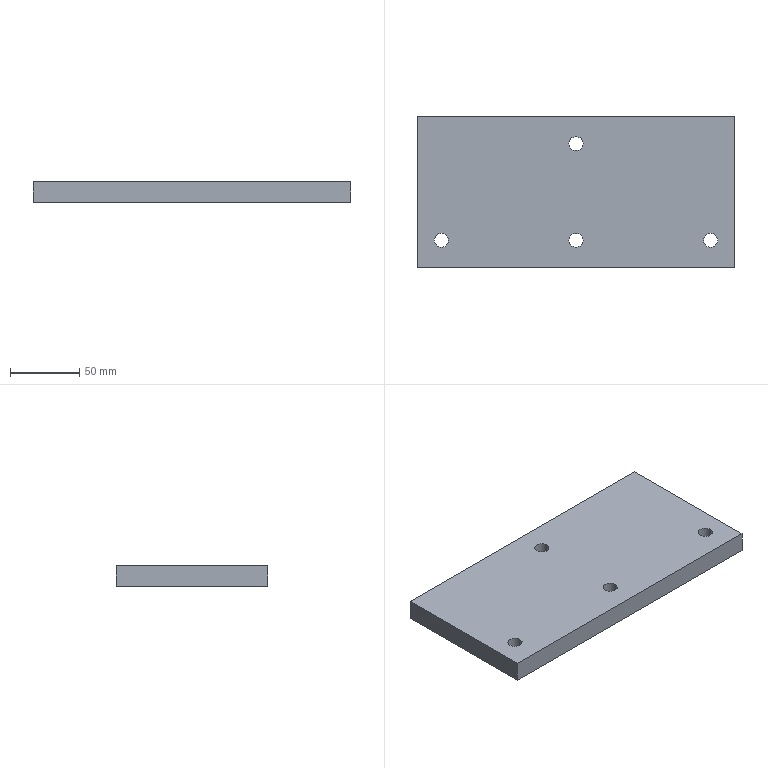Part | SolidWorks | features Extrusion 1, HoleWzd 1 | 1 solid | 14 faces | box 230 x 110 x 15 mm | volume 374597 mm3 | cylinder 8 | plane 6 | commonest cylinder face diameters 10.2 x8
STEP:
#1=CARTESIAN_POINT('',(-102.6,-35.,0.));
#2=VERTEX_POINT('',#1);
#3=CARTESIAN_POINT('',(-92.4,-35.,0.));
#4=VERTEX_POINT('',#3);
#5=CARTESIAN_POINT('',(-97.5,-35.,0.));
#6=DIRECTION('',(0.,0.,1.));
#7=DIRECTION('',(1.,0.,0.));
#8=AXIS2_PLACEMENT_3D('',#5,#6,#7);
#9=CIRCLE('',#8,5.1);
#10=EDGE_CURVE('',#2,#4,#9,.T.);
#11=ORIENTED_EDGE('',*,*,#10,.F.);
#12=CARTESIAN_POINT('',(-102.6,-35.,15.));
#13=VERTEX_POINT('',#12);
#14=CARTESIAN_POINT('',(-102.6,-35.,15.));
#15=DIRECTION('',(0.,0.,1.));
#16=VECTOR('',#15,1000.);
#17=LINE('',#14,#16);
#18=EDGE_CURVE('',#2,#13,#17,.T.);
#19=ORIENTED_EDGE('',*,*,#18,.T.);
#20=CARTESIAN_POINT('',(-92.4,-35.,15.));
#21=VERTEX_POINT('',#20);
#22=CARTESIAN_POINT('',(-97.5,-35.,15.));
#23=DIRECTION('',(0.,0.,1.));
#24=DIRECTION('',(1.,0.,0.));
#25=AXIS2_PLACEMENT_3D('',#22,#23,#24);
#26=CIRCLE('',#25,5.1);
#27=EDGE_CURVE('',#13,#21,#26,.T.);
#28=ORIENTED_EDGE('',*,*,#27,.T.);
#29=CARTESIAN_POINT('',(-92.4,-35.,15.));
#30=DIRECTION('',(0.,0.,1.));
#31=VECTOR('',#30,1000.);
#32=LINE('',#29,#31);
#33=EDGE_CURVE('',#4,#21,#32,.T.);
#34=ORIENTED_EDGE('',*,*,#33,.F.);
#35=EDGE_LOOP('',(#11,#19,#28,#34));
#36=FACE_OUTER_BOUND('',#35,.T.);
#37=CARTESIAN_POINT('',(-97.5,-35.,15.));
#38=DIRECTION('',(0.,0.,1.));
#39=DIRECTION('',(1.,0.,0.));
#40=AXIS2_PLACEMENT_3D('',#37,#38,#39);
#41=CYLINDRICAL_SURFACE('',#40,5.1);
#42=ADVANCED_FACE('',(#36),#41,.F.);
#43=CARTESIAN_POINT('',(92.4,-35.,0.));
#44=VERTEX_POINT('',#43);
#45=CARTESIAN_POINT('',(102.6,-35.,0.));
#46=VERTEX_POINT('',#45);
#47=CARTESIAN_POINT('',(97.5,-35.,0.));
#48=DIRECTION('',(0.,0.,1.));
#49=DIRECTION('',(1.,0.,0.));
#50=AXIS2_PLACEMENT_3D('',#47,#48,#49);
#51=CIRCLE('',#50,5.1);
#52=EDGE_CURVE('',#44,#46,#51,.T.);
#53=ORIENTED_EDGE('',*,*,#52,.F.);
#54=CARTESIAN_POINT('',(92.4,-35.,15.));
#55=VERTEX_POINT('',#54);
#56=CARTESIAN_POINT('',(92.4,-35.,15.));
#57=DIRECTION('',(0.,0.,1.));
#58=VECTOR('',#57,1000.);
#59=LINE('',#56,#58);
#60=EDGE_CURVE('',#44,#55,#59,.T.);
#61=ORIENTED_EDGE('',*,*,#60,.T.);
#62=CARTESIAN_POINT('',(102.6,-35.,15.));
#63=VERTEX_POINT('',#62);
#64=CARTESIAN_POINT('',(97.5,-35.,15.));
#65=DIRECTION('',(0.,0.,1.));
#66=DIRECTION('',(1.,0.,0.));
#67=AXIS2_PLACEMENT_3D('',#64,#65,#66);
#68=CIRCLE('',#67,5.1);
#69=EDGE_CURVE('',#55,#63,#68,.T.);
#70=ORIENTED_EDGE('',*,*,#69,.T.);
#71=CARTESIAN_POINT('',(102.6,-35.,15.));
#72=DIRECTION('',(0.,0.,1.));
#73=VECTOR('',#72,1000.);
#74=LINE('',#71,#73);
#75=EDGE_CURVE('',#46,#63,#74,.T.);
#76=ORIENTED_EDGE('',*,*,#75,.F.);
#77=EDGE_LOOP('',(#53,#61,#70,#76));
#78=FACE_OUTER_BOUND('',#77,.T.);
#79=CARTESIAN_POINT('',(97.5,-35.,15.));
#80=DIRECTION('',(0.,0.,1.));
#81=DIRECTION('',(1.,0.,0.));
#82=AXIS2_PLACEMENT_3D('',#79,#80,#81);
#83=CYLINDRICAL_SURFACE('',#82,5.1);
#84=ADVANCED_FACE('',(#78),#83,.F.);
#85=CARTESIAN_POINT('',(-5.1,35.,0.));
#86=VERTEX_POINT('',#85);
#87=CARTESIAN_POINT('',(5.1,35.,0.));
#88=VERTEX_POINT('',#87);
#89=CARTESIAN_POINT('',(0.,35.,0.));
#90=DIRECTION('',(0.,0.,1.));
#91=DIRECTION('',(1.,0.,0.));
#92=AXIS2_PLACEMENT_3D('',#89,#90,#91);
#93=CIRCLE('',#92,5.1);
#94=EDGE_CURVE('',#86,#88,#93,.T.);
#95=ORIENTED_EDGE('',*,*,#94,.F.);
#96=CARTESIAN_POINT('',(-5.1,35.,15.));
#97=VERTEX_POINT('',#96);
#98=CARTESIAN_POINT('',(-5.1,35.,15.));
#99=DIRECTION('',(0.,0.,1.));
#100=VECTOR('',#99,1000.);
#101=LINE('',#98,#100);
#102=EDGE_CURVE('',#86,#97,#101,.T.);
#103=ORIENTED_EDGE('',*,*,#102,.T.);
#104=CARTESIAN_POINT('',(5.1,35.,15.));
#105=VERTEX_POINT('',#104);
#106=CARTESIAN_POINT('',(0.,35.,15.));
#107=DIRECTION('',(0.,0.,1.));
#108=DIRECTION('',(1.,0.,0.));
#109=AXIS2_PLACEMENT_3D('',#106,#107,#108);
#110=CIRCLE('',#109,5.1);
#111=EDGE_CURVE('',#97,#105,#110,.T.);
#112=ORIENTED_EDGE('',*,*,#111,.T.);
#113=CARTESIAN_POINT('',(5.1,35.,15.));
#114=DIRECTION('',(0.,0.,1.));
#115=VECTOR('',#114,1000.);
#116=LINE('',#113,#115);
#117=EDGE_CURVE('',#88,#105,#116,.T.);
#118=ORIENTED_EDGE('',*,*,#117,.F.);
#119=EDGE_LOOP('',(#95,#103,#112,#118));
#120=FACE_OUTER_BOUND('',#119,.T.);
#121=CARTESIAN_POINT('',(0.,35.,15.));
#122=DIRECTION('',(0.,0.,1.));
#123=DIRECTION('',(1.,0.,0.));
#124=AXIS2_PLACEMENT_3D('',#121,#122,#123);
#125=CYLINDRICAL_SURFACE('',#124,5.1);
#126=ADVANCED_FACE('',(#120),#125,.F.);
#127=CARTESIAN_POINT('',(-5.1,-35.,0.));
#128=VERTEX_POINT('',#127);
#129=CARTESIAN_POINT('',(5.1,-35.,0.));
#130=VERTEX_POINT('',#129);
#131=CARTESIAN_POINT('',(0.,-35.,0.));
#132=DIRECTION('',(0.,0.,1.));
#133=DIRECTION('',(1.,0.,0.));
#134=AXIS2_PLACEMENT_3D('',#131,#132,#133);
#135=CIRCLE('',#134,5.1);
#136=EDGE_CURVE('',#128,#130,#135,.T.);
#137=ORIENTED_EDGE('',*,*,#136,.F.);
#138=CARTESIAN_POINT('',(-5.1,-35.,15.));
#139=VERTEX_POINT('',#138);
#140=CARTESIAN_POINT('',(-5.1,-35.,15.));
#141=DIRECTION('',(0.,0.,1.));
#142=VECTOR('',#141,1000.);
#143=LINE('',#140,#142);
#144=EDGE_CURVE('',#128,#139,#143,.T.);
#145=ORIENTED_EDGE('',*,*,#144,.T.);
#146=CARTESIAN_POINT('',(5.1,-35.,15.));
#147=VERTEX_POINT('',#146);
#148=CARTESIAN_POINT('',(0.,-35.,15.));
#149=DIRECTION('',(0.,0.,1.));
#150=DIRECTION('',(1.,0.,0.));
#151=AXIS2_PLACEMENT_3D('',#148,#149,#150);
#152=CIRCLE('',#151,5.1);
#153=EDGE_CURVE('',#139,#147,#152,.T.);
#154=ORIENTED_EDGE('',*,*,#153,.T.);
#155=CARTESIAN_POINT('',(5.1,-35.,15.));
#156=DIRECTION('',(0.,0.,1.));
#157=VECTOR('',#156,1000.);
#158=LINE('',#155,#157);
#159=EDGE_CURVE('',#130,#147,#158,.T.);
#160=ORIENTED_EDGE('',*,*,#159,.F.);
#161=EDGE_LOOP('',(#137,#145,#154,#160));
#162=FACE_OUTER_BOUND('',#161,.T.);
#163=CARTESIAN_POINT('',(0.,-35.,15.));
#164=DIRECTION('',(0.,0.,1.));
#165=DIRECTION('',(1.,0.,0.));
#166=AXIS2_PLACEMENT_3D('',#163,#164,#165);
#167=CYLINDRICAL_SURFACE('',#166,5.1);
#168=ADVANCED_FACE('',(#162),#167,.F.);
#169=CARTESIAN_POINT('',(115.,-55.,0.));
#170=VERTEX_POINT('',#169);
#171=CARTESIAN_POINT('',(115.,55.,0.));
#172=VERTEX_POINT('',#171);
#173=CARTESIAN_POINT('',(115.,55.,0.));
#174=DIRECTION('',(0.,1.,0.));
#175=VECTOR('',#174,1000.);
#176=LINE('',#173,#175);
#177=EDGE_CURVE('',#170,#172,#176,.T.);
#178=ORIENTED_EDGE('',*,*,#177,.T.);
#179=CARTESIAN_POINT('',(115.,55.,15.));
#180=VERTEX_POINT('',#179);
#181=CARTESIAN_POINT('',(115.,55.,15.));
#182=DIRECTION('',(0.,0.,-1.));
#183=VECTOR('',#182,1000.);
#184=LINE('',#181,#183);
#185=EDGE_CURVE('',#180,#172,#184,.T.);
#186=ORIENTED_EDGE('',*,*,#185,.F.);
#187=CARTESIAN_POINT('',(115.,-55.,15.));
#188=VERTEX_POINT('',#187);
#189=CARTESIAN_POINT('',(115.,55.,15.));
#190=DIRECTION('',(0.,1.,0.));
#191=VECTOR('',#190,1000.);
#192=LINE('',#189,#191);
#193=EDGE_CURVE('',#188,#180,#192,.T.);
#194=ORIENTED_EDGE('',*,*,#193,.F.);
#195=CARTESIAN_POINT('',(115.,-55.,15.));
#196=DIRECTION('',(0.,0.,-1.));
#197=VECTOR('',#196,1000.);
#198=LINE('',#195,#197);
#199=EDGE_CURVE('',#188,#170,#198,.T.);
#200=ORIENTED_EDGE('',*,*,#199,.T.);
#201=EDGE_LOOP('',(#178,#186,#194,#200));
#202=FACE_OUTER_BOUND('',#201,.T.);
#203=CARTESIAN_POINT('',(115.,55.,15.));
#204=DIRECTION('',(-1.,0.,0.));
#205=DIRECTION('',(0.,0.,1.));
#206=AXIS2_PLACEMENT_3D('',#203,#204,#205);
#207=PLANE('',#206);
#208=ADVANCED_FACE('',(#202),#207,.F.);
#209=CARTESIAN_POINT('',(-115.,55.,0.));
#210=VERTEX_POINT('',#209);
#211=CARTESIAN_POINT('',(-115.,55.,0.));
#212=DIRECTION('',(-1.,0.,0.));
#213=VECTOR('',#212,1000.);
#214=LINE('',#211,#213);
#215=EDGE_CURVE('',#172,#210,#214,.T.);
#216=ORIENTED_EDGE('',*,*,#215,.T.);
#217=CARTESIAN_POINT('',(-115.,55.,15.));
#218=VERTEX_POINT('',#217);
#219=CARTESIAN_POINT('',(-115.,55.,15.));
#220=DIRECTION('',(0.,0.,-1.));
#221=VECTOR('',#220,1000.);
#222=LINE('',#219,#221);
#223=EDGE_CURVE('',#218,#210,#222,.T.);
#224=ORIENTED_EDGE('',*,*,#223,.F.);
#225=CARTESIAN_POINT('',(-115.,55.,15.));
#226=DIRECTION('',(-1.,0.,0.));
#227=VECTOR('',#226,1000.);
#228=LINE('',#225,#227);
#229=EDGE_CURVE('',#180,#218,#228,.T.);
#230=ORIENTED_EDGE('',*,*,#229,.F.);
#231=ORIENTED_EDGE('',*,*,#185,.T.);
#232=EDGE_LOOP('',(#216,#224,#230,#231));
#233=FACE_OUTER_BOUND('',#232,.T.);
#234=CARTESIAN_POINT('',(-115.,55.,15.));
#235=DIRECTION('',(0.,-1.,0.));
#236=DIRECTION('',(0.,0.,-1.));
#237=AXIS2_PLACEMENT_3D('',#234,#235,#236);
#238=PLANE('',#237);
#239=ADVANCED_FACE('',(#233),#238,.F.);
#240=CARTESIAN_POINT('',(-115.,-55.,0.));
#241=VERTEX_POINT('',#240);
#242=CARTESIAN_POINT('',(-115.,55.,0.));
#243=DIRECTION('',(0.,-1.,0.));
#244=VECTOR('',#243,1000.);
#245=LINE('',#242,#244);
#246=EDGE_CURVE('',#210,#241,#245,.T.);
#247=ORIENTED_EDGE('',*,*,#246,.T.);
#248=CARTESIAN_POINT('',(-115.,-55.,15.));
#249=VERTEX_POINT('',#248);
#250=CARTESIAN_POINT('',(-115.,-55.,15.));
#251=DIRECTION('',(0.,0.,-1.));
#252=VECTOR('',#251,1000.);
#253=LINE('',#250,#252);
#254=EDGE_CURVE('',#249,#241,#253,.T.);
#255=ORIENTED_EDGE('',*,*,#254,.F.);
#256=CARTESIAN_POINT('',(-115.,55.,15.));
#257=DIRECTION('',(0.,-1.,0.));
#258=VECTOR('',#257,1000.);
#259=LINE('',#256,#258);
#260=EDGE_CURVE('',#218,#249,#259,.T.);
#261=ORIENTED_EDGE('',*,*,#260,.F.);
#262=ORIENTED_EDGE('',*,*,#223,.T.);
#263=EDGE_LOOP('',(#247,#255,#261,#262));
#264=FACE_OUTER_BOUND('',#263,.T.);
#265=CARTESIAN_POINT('',(-115.,55.,15.));
#266=DIRECTION('',(1.,0.,0.));
#267=DIRECTION('',(0.,1.,0.));
#268=AXIS2_PLACEMENT_3D('',#265,#266,#267);
#269=PLANE('',#268);
#270=ADVANCED_FACE('',(#264),#269,.F.);
#271=CARTESIAN_POINT('',(-115.,-55.,0.));
#272=DIRECTION('',(1.,0.,0.));
#273=VECTOR('',#272,1000.);
#274=LINE('',#271,#273);
#275=EDGE_CURVE('',#241,#170,#274,.T.);
#276=ORIENTED_EDGE('',*,*,#275,.T.);
#277=ORIENTED_EDGE('',*,*,#199,.F.);
#278=CARTESIAN_POINT('',(-115.,-55.,15.));
#279=DIRECTION('',(1.,0.,0.));
#280=VECTOR('',#279,1000.);
#281=LINE('',#278,#280);
#282=EDGE_CURVE('',#249,#188,#281,.T.);
#283=ORIENTED_EDGE('',*,*,#282,.F.);
#284=ORIENTED_EDGE('',*,*,#254,.T.);
#285=EDGE_LOOP('',(#276,#277,#283,#284));
#286=FACE_OUTER_BOUND('',#285,.T.);
#287=CARTESIAN_POINT('',(-115.,-55.,15.));
#288=DIRECTION('',(0.,1.,0.));
#289=DIRECTION('',(0.,0.,1.));
#290=AXIS2_PLACEMENT_3D('',#287,#288,#289);
#291=PLANE('',#290);
#292=ADVANCED_FACE('',(#286),#291,.F.);
#293=CARTESIAN_POINT('',(-97.5,-35.,15.));
#294=DIRECTION('',(0.,0.,1.));
#295=DIRECTION('',(1.,0.,0.));
#296=AXIS2_PLACEMENT_3D('',#293,#294,#295);
#297=CIRCLE('',#296,5.1);
#298=EDGE_CURVE('',#21,#13,#297,.T.);
#299=ORIENTED_EDGE('',*,*,#298,.F.);
#300=ORIENTED_EDGE('',*,*,#27,.F.);
#301=EDGE_LOOP('',(#299,#300));
#302=FACE_BOUND('',#301,.T.);
#303=CARTESIAN_POINT('',(97.5,-35.,15.));
#304=DIRECTION('',(0.,0.,1.));
#305=DIRECTION('',(1.,0.,0.));
#306=AXIS2_PLACEMENT_3D('',#303,#304,#305);
#307=CIRCLE('',#306,5.1);
#308=EDGE_CURVE('',#63,#55,#307,.T.);
#309=ORIENTED_EDGE('',*,*,#308,.F.);
#310=ORIENTED_EDGE('',*,*,#69,.F.);
#311=EDGE_LOOP('',(#309,#310));
#312=FACE_BOUND('',#311,.T.);
#313=CARTESIAN_POINT('',(0.,35.,15.));
#314=DIRECTION('',(0.,0.,1.));
#315=DIRECTION('',(1.,0.,0.));
#316=AXIS2_PLACEMENT_3D('',#313,#314,#315);
#317=CIRCLE('',#316,5.1);
#318=EDGE_CURVE('',#105,#97,#317,.T.);
#319=ORIENTED_EDGE('',*,*,#318,.F.);
#320=ORIENTED_EDGE('',*,*,#111,.F.);
#321=EDGE_LOOP('',(#319,#320));
#322=FACE_BOUND('',#321,.T.);
#323=CARTESIAN_POINT('',(0.,-35.,15.));
#324=DIRECTION('',(0.,0.,1.));
#325=DIRECTION('',(1.,0.,0.));
#326=AXIS2_PLACEMENT_3D('',#323,#324,#325);
#327=CIRCLE('',#326,5.1);
#328=EDGE_CURVE('',#147,#139,#327,.T.);
#329=ORIENTED_EDGE('',*,*,#328,.F.);
#330=ORIENTED_EDGE('',*,*,#153,.F.);
#331=EDGE_LOOP('',(#329,#330));
#332=FACE_BOUND('',#331,.T.);
#333=ORIENTED_EDGE('',*,*,#193,.T.);
#334=ORIENTED_EDGE('',*,*,#229,.T.);
#335=ORIENTED_EDGE('',*,*,#260,.T.);
#336=ORIENTED_EDGE('',*,*,#282,.T.);
#337=EDGE_LOOP('',(#333,#334,#335,#336));
#338=FACE_OUTER_BOUND('',#337,.T.);
#339=CARTESIAN_POINT('',(0.,0.,15.));
#340=DIRECTION('',(0.,0.,1.));
#341=DIRECTION('',(1.,0.,0.));
#342=AXIS2_PLACEMENT_3D('',#339,#340,#341);
#343=PLANE('',#342);
#344=ADVANCED_FACE('',(#302,#312,#322,#332,#338),#343,.T.);
#345=CARTESIAN_POINT('',(-97.5,-35.,0.));
#346=DIRECTION('',(0.,0.,1.));
#347=DIRECTION('',(1.,0.,0.));
#348=AXIS2_PLACEMENT_3D('',#345,#346,#347);
#349=CIRCLE('',#348,5.1);
#350=EDGE_CURVE('',#4,#2,#349,.T.);
#351=ORIENTED_EDGE('',*,*,#350,.T.);
#352=ORIENTED_EDGE('',*,*,#10,.T.);
#353=EDGE_LOOP('',(#351,#352));
#354=FACE_BOUND('',#353,.T.);
#355=CARTESIAN_POINT('',(97.5,-35.,0.));
#356=DIRECTION('',(0.,0.,1.));
#357=DIRECTION('',(1.,0.,0.));
#358=AXIS2_PLACEMENT_3D('',#355,#356,#357);
#359=CIRCLE('',#358,5.1);
#360=EDGE_CURVE('',#46,#44,#359,.T.);
#361=ORIENTED_EDGE('',*,*,#360,.T.);
#362=ORIENTED_EDGE('',*,*,#52,.T.);
#363=EDGE_LOOP('',(#361,#362));
#364=FACE_BOUND('',#363,.T.);
#365=CARTESIAN_POINT('',(0.,35.,0.));
#366=DIRECTION('',(0.,0.,1.));
#367=DIRECTION('',(1.,0.,0.));
#368=AXIS2_PLACEMENT_3D('',#365,#366,#367);
#369=CIRCLE('',#368,5.1);
#370=EDGE_CURVE('',#88,#86,#369,.T.);
#371=ORIENTED_EDGE('',*,*,#370,.T.);
#372=ORIENTED_EDGE('',*,*,#94,.T.);
#373=EDGE_LOOP('',(#371,#372));
#374=FACE_BOUND('',#373,.T.);
#375=CARTESIAN_POINT('',(0.,-35.,0.));
#376=DIRECTION('',(0.,0.,1.));
#377=DIRECTION('',(1.,0.,0.));
#378=AXIS2_PLACEMENT_3D('',#375,#376,#377);
#379=CIRCLE('',#378,5.1);
#380=EDGE_CURVE('',#130,#128,#379,.T.);
#381=ORIENTED_EDGE('',*,*,#380,.T.);
#382=ORIENTED_EDGE('',*,*,#136,.T.);
#383=EDGE_LOOP('',(#381,#382));
#384=FACE_BOUND('',#383,.T.);
#385=ORIENTED_EDGE('',*,*,#177,.F.);
#386=ORIENTED_EDGE('',*,*,#275,.F.);
#387=ORIENTED_EDGE('',*,*,#246,.F.);
#388=ORIENTED_EDGE('',*,*,#215,.F.);
#389=EDGE_LOOP('',(#385,#386,#387,#388));
#390=FACE_OUTER_BOUND('',#389,.T.);
#391=CARTESIAN_POINT('',(0.,0.,0.));
#392=DIRECTION('',(0.,0.,1.));
#393=DIRECTION('',(1.,0.,0.));
#394=AXIS2_PLACEMENT_3D('',#391,#392,#393);
#395=PLANE('',#394);
#396=ADVANCED_FACE('',(#354,#364,#374,#384,#390),#395,.F.);
#397=ORIENTED_EDGE('',*,*,#144,.F.);
#398=ORIENTED_EDGE('',*,*,#380,.F.);
#399=ORIENTED_EDGE('',*,*,#159,.T.);
#400=ORIENTED_EDGE('',*,*,#328,.T.);
#401=EDGE_LOOP('',(#397,#398,#399,#400));
#402=FACE_OUTER_BOUND('',#401,.T.);
#403=CARTESIAN_POINT('',(0.,-35.,15.));
#404=DIRECTION('',(0.,0.,1.));
#405=DIRECTION('',(1.,0.,0.));
#406=AXIS2_PLACEMENT_3D('',#403,#404,#405);
#407=CYLINDRICAL_SURFACE('',#406,5.1);
#408=ADVANCED_FACE('',(#402),#407,.F.);
#409=ORIENTED_EDGE('',*,*,#102,.F.);
#410=ORIENTED_EDGE('',*,*,#370,.F.);
#411=ORIENTED_EDGE('',*,*,#117,.T.);
#412=ORIENTED_EDGE('',*,*,#318,.T.);
#413=EDGE_LOOP('',(#409,#410,#411,#412));
#414=FACE_OUTER_BOUND('',#413,.T.);
#415=CARTESIAN_POINT('',(0.,35.,15.));
#416=DIRECTION('',(0.,0.,1.));
#417=DIRECTION('',(1.,0.,0.));
#418=AXIS2_PLACEMENT_3D('',#415,#416,#417);
#419=CYLINDRICAL_SURFACE('',#418,5.1);
#420=ADVANCED_FACE('',(#414),#419,.F.);
#421=ORIENTED_EDGE('',*,*,#60,.F.);
#422=ORIENTED_EDGE('',*,*,#360,.F.);
#423=ORIENTED_EDGE('',*,*,#75,.T.);
#424=ORIENTED_EDGE('',*,*,#308,.T.);
#425=EDGE_LOOP('',(#421,#422,#423,#424));
#426=FACE_OUTER_BOUND('',#425,.T.);
#427=CARTESIAN_POINT('',(97.5,-35.,15.));
#428=DIRECTION('',(0.,0.,1.));
#429=DIRECTION('',(1.,0.,0.));
#430=AXIS2_PLACEMENT_3D('',#427,#428,#429);
#431=CYLINDRICAL_SURFACE('',#430,5.1);
#432=ADVANCED_FACE('',(#426),#431,.F.);
#433=ORIENTED_EDGE('',*,*,#18,.F.);
#434=ORIENTED_EDGE('',*,*,#350,.F.);
#435=ORIENTED_EDGE('',*,*,#33,.T.);
#436=ORIENTED_EDGE('',*,*,#298,.T.);
#437=EDGE_LOOP('',(#433,#434,#435,#436));
#438=FACE_OUTER_BOUND('',#437,.T.);
#439=CARTESIAN_POINT('',(-97.5,-35.,15.));
#440=DIRECTION('',(0.,0.,1.));
#441=DIRECTION('',(1.,0.,0.));
#442=AXIS2_PLACEMENT_3D('',#439,#440,#441);
#443=CYLINDRICAL_SURFACE('',#442,5.1);
#444=ADVANCED_FACE('',(#438),#443,.F.);
#445=CLOSED_SHELL('',(#42,#84,#126,#168,#208,#239,#270,#292,#344,#396,#408,#420,#432,#444));
#446=MANIFOLD_SOLID_BREP('',#445);
#447=CARTESIAN_POINT('',(0.,0.,0.));
#448=DIRECTION('',(0.,0.,1.));
#449=DIRECTION('',(1.,0.,0.));
#450=AXIS2_PLACEMENT_3D('',#447,#448,#449);
#451=(LENGTH_UNIT()NAMED_UNIT(*)SI_UNIT(.MILLI.,.METRE.));
#452=UNCERTAINTY_MEASURE_WITH_UNIT(LENGTH_MEASURE(0.00001),#451,'','');
#453=(NAMED_UNIT(*)PLANE_ANGLE_UNIT()SI_UNIT($,.RADIAN.));
#454=(NAMED_UNIT(*)SI_UNIT($,.STERADIAN.)SOLID_ANGLE_UNIT());
#455=(GEOMETRIC_REPRESENTATION_CONTEXT(3)GLOBAL_UNCERTAINTY_ASSIGNED_CONTEXT((#452))GLOBAL_UNIT_ASSIGNED_CONTEXT((#451,#453,#454))REPRESENTATION_CONTEXT('',''));
#456=ADVANCED_BREP_SHAPE_REPRESENTATION('',(#446,#450),#455);